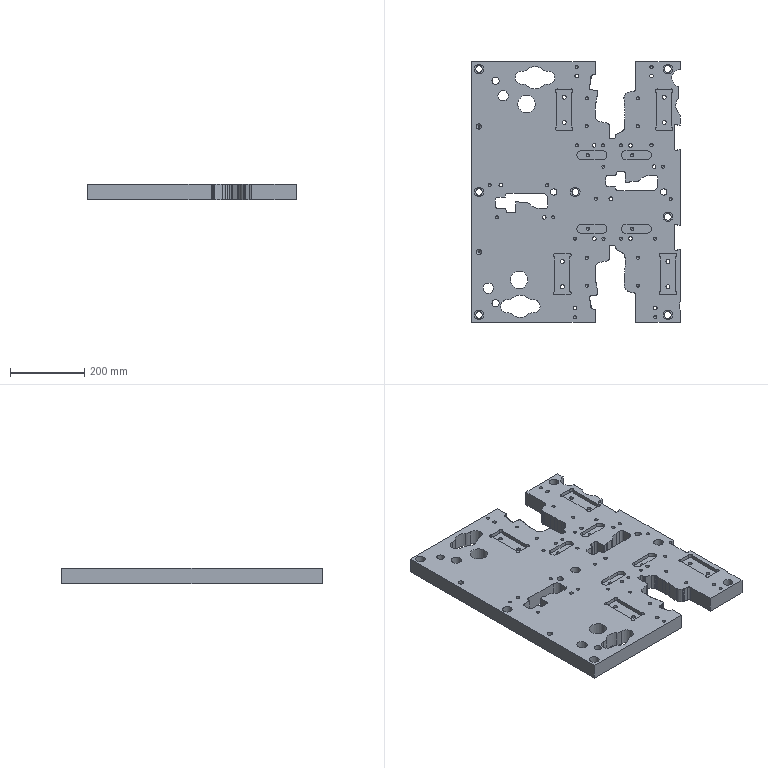Part | STEP file | lll_id3918_x_t | 1 solid | 446 faces | box 564.041 x 704 x 42 mm | volume 13422276 mm3 | cylinder 298 | plane 114 | cone 34 | commonest cylinder face diameters 10 x32 8.506 x28 25 x20 40 x11 11 x10 1 x8